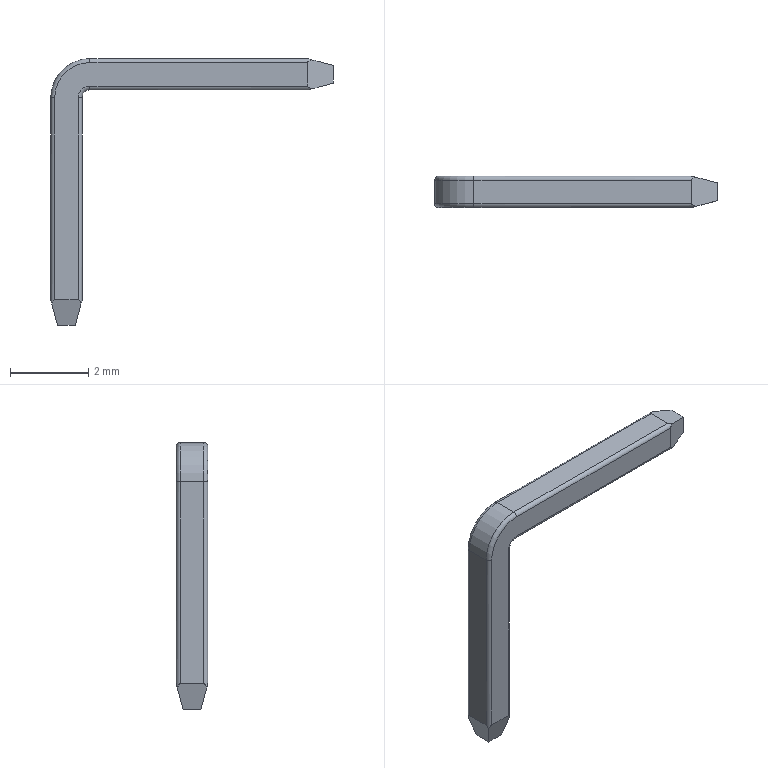Part | STEP file | RJ-USIO-V1_2-220411_14 | 1 solid | 30 faces | box 7.2 x 0.8 x 6.8 mm | volume 7.87 mm3 | plane 16 | cylinder 10 | torus 4 | commonest cylinder face diameters 0.2 x8 0.4 x1 2 x1